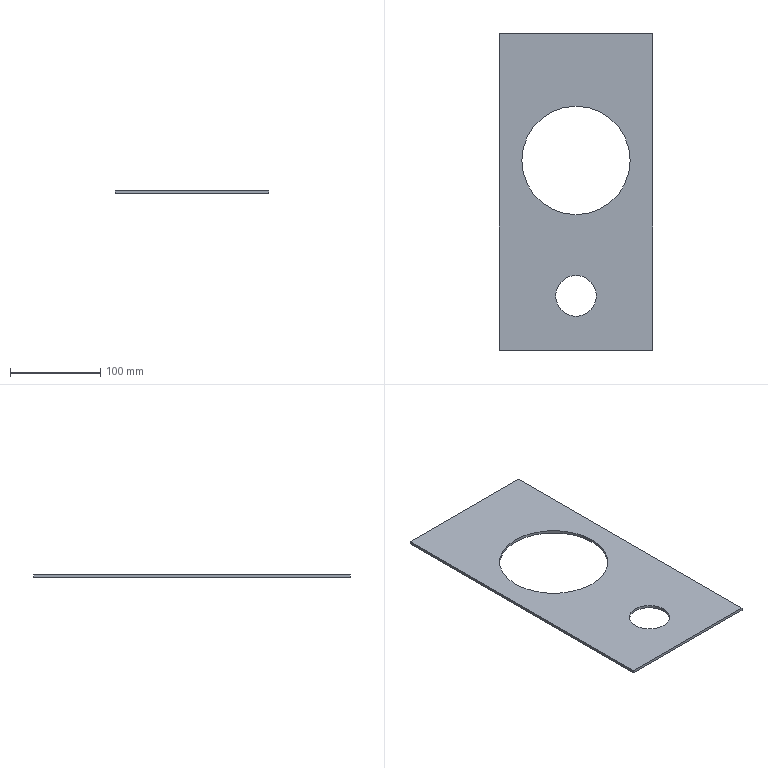Part | SolidWorks | features Extrusion 1 | 1 solid | 10 faces | box 170 x 350 x 3 mm | volume 139800 mm3 | plane 6 | cylinder 4 | commonest cylinder face diameters 45 x2 120 x2
STEP:
#1=CARTESIAN_POINT('',(62.5,60.,3.));
#2=VERTEX_POINT('',#1);
#3=CARTESIAN_POINT('',(107.5,60.,3.));
#4=VERTEX_POINT('',#3);
#5=CARTESIAN_POINT('',(85.,60.,3.));
#6=DIRECTION('',(0.,0.,1.));
#7=DIRECTION('',(1.,0.,0.));
#8=AXIS2_PLACEMENT_3D('',#5,#6,#7);
#9=CIRCLE('',#8,22.5);
#10=EDGE_CURVE('',#2,#4,#9,.T.);
#11=ORIENTED_EDGE('',*,*,#10,.T.);
#12=CARTESIAN_POINT('',(107.5,60.,0.));
#13=VERTEX_POINT('',#12);
#14=CARTESIAN_POINT('',(107.5,60.,3.));
#15=DIRECTION('',(0.,0.,-1.));
#16=VECTOR('',#15,1000.);
#17=LINE('',#14,#16);
#18=EDGE_CURVE('',#4,#13,#17,.T.);
#19=ORIENTED_EDGE('',*,*,#18,.T.);
#20=CARTESIAN_POINT('',(62.5,60.,0.));
#21=VERTEX_POINT('',#20);
#22=CARTESIAN_POINT('',(85.,60.,0.));
#23=DIRECTION('',(0.,0.,1.));
#24=DIRECTION('',(1.,0.,0.));
#25=AXIS2_PLACEMENT_3D('',#22,#23,#24);
#26=CIRCLE('',#25,22.5);
#27=EDGE_CURVE('',#21,#13,#26,.T.);
#28=ORIENTED_EDGE('',*,*,#27,.F.);
#29=CARTESIAN_POINT('',(62.5,60.,3.));
#30=DIRECTION('',(0.,0.,-1.));
#31=VECTOR('',#30,1000.);
#32=LINE('',#29,#31);
#33=EDGE_CURVE('',#2,#21,#32,.T.);
#34=ORIENTED_EDGE('',*,*,#33,.F.);
#35=EDGE_LOOP('',(#11,#19,#28,#34));
#36=FACE_OUTER_BOUND('',#35,.T.);
#37=CARTESIAN_POINT('',(85.,60.,3.));
#38=DIRECTION('',(0.,0.,-1.));
#39=DIRECTION('',(-1.,0.,0.));
#40=AXIS2_PLACEMENT_3D('',#37,#38,#39);
#41=CYLINDRICAL_SURFACE('',#40,22.5);
#42=ADVANCED_FACE('',(#36),#41,.F.);
#43=CARTESIAN_POINT('',(25.,210.,3.));
#44=VERTEX_POINT('',#43);
#45=CARTESIAN_POINT('',(145.,210.,3.));
#46=VERTEX_POINT('',#45);
#47=CARTESIAN_POINT('',(85.,210.,3.));
#48=DIRECTION('',(0.,0.,1.));
#49=DIRECTION('',(1.,0.,0.));
#50=AXIS2_PLACEMENT_3D('',#47,#48,#49);
#51=CIRCLE('',#50,60.);
#52=EDGE_CURVE('',#44,#46,#51,.T.);
#53=ORIENTED_EDGE('',*,*,#52,.T.);
#54=CARTESIAN_POINT('',(145.,210.,0.));
#55=VERTEX_POINT('',#54);
#56=CARTESIAN_POINT('',(145.,210.,3.));
#57=DIRECTION('',(0.,0.,-1.));
#58=VECTOR('',#57,1000.);
#59=LINE('',#56,#58);
#60=EDGE_CURVE('',#46,#55,#59,.T.);
#61=ORIENTED_EDGE('',*,*,#60,.T.);
#62=CARTESIAN_POINT('',(25.,210.,0.));
#63=VERTEX_POINT('',#62);
#64=CARTESIAN_POINT('',(85.,210.,0.));
#65=DIRECTION('',(0.,0.,1.));
#66=DIRECTION('',(1.,0.,0.));
#67=AXIS2_PLACEMENT_3D('',#64,#65,#66);
#68=CIRCLE('',#67,60.);
#69=EDGE_CURVE('',#63,#55,#68,.T.);
#70=ORIENTED_EDGE('',*,*,#69,.F.);
#71=CARTESIAN_POINT('',(25.,210.,3.));
#72=DIRECTION('',(0.,0.,-1.));
#73=VECTOR('',#72,1000.);
#74=LINE('',#71,#73);
#75=EDGE_CURVE('',#44,#63,#74,.T.);
#76=ORIENTED_EDGE('',*,*,#75,.F.);
#77=EDGE_LOOP('',(#53,#61,#70,#76));
#78=FACE_OUTER_BOUND('',#77,.T.);
#79=CARTESIAN_POINT('',(85.,210.,3.));
#80=DIRECTION('',(0.,0.,-1.));
#81=DIRECTION('',(-1.,0.,0.));
#82=AXIS2_PLACEMENT_3D('',#79,#80,#81);
#83=CYLINDRICAL_SURFACE('',#82,60.);
#84=ADVANCED_FACE('',(#78),#83,.F.);
#85=ORIENTED_EDGE('',*,*,#52,.F.);
#86=CARTESIAN_POINT('',(85.,210.,3.));
#87=DIRECTION('',(0.,0.,1.));
#88=DIRECTION('',(1.,0.,0.));
#89=AXIS2_PLACEMENT_3D('',#86,#87,#88);
#90=CIRCLE('',#89,60.);
#91=EDGE_CURVE('',#46,#44,#90,.T.);
#92=ORIENTED_EDGE('',*,*,#91,.F.);
#93=EDGE_LOOP('',(#85,#92));
#94=FACE_BOUND('',#93,.T.);
#95=CARTESIAN_POINT('',(0.,350.,3.));
#96=VERTEX_POINT('',#95);
#97=CARTESIAN_POINT('',(0.,0.,3.));
#98=VERTEX_POINT('',#97);
#99=CARTESIAN_POINT('',(0.,0.,3.));
#100=DIRECTION('',(0.,-1.,0.));
#101=VECTOR('',#100,1000.);
#102=LINE('',#99,#101);
#103=EDGE_CURVE('',#96,#98,#102,.T.);
#104=ORIENTED_EDGE('',*,*,#103,.T.);
#105=CARTESIAN_POINT('',(170.,0.,3.));
#106=VERTEX_POINT('',#105);
#107=CARTESIAN_POINT('',(0.,0.,3.));
#108=DIRECTION('',(1.,0.,0.));
#109=VECTOR('',#108,1000.);
#110=LINE('',#107,#109);
#111=EDGE_CURVE('',#98,#106,#110,.T.);
#112=ORIENTED_EDGE('',*,*,#111,.T.);
#113=CARTESIAN_POINT('',(170.,350.,3.));
#114=VERTEX_POINT('',#113);
#115=CARTESIAN_POINT('',(170.,0.,3.));
#116=DIRECTION('',(0.,1.,0.));
#117=VECTOR('',#116,1000.);
#118=LINE('',#115,#117);
#119=EDGE_CURVE('',#106,#114,#118,.T.);
#120=ORIENTED_EDGE('',*,*,#119,.T.);
#121=CARTESIAN_POINT('',(0.,350.,3.));
#122=DIRECTION('',(-1.,0.,0.));
#123=VECTOR('',#122,1000.);
#124=LINE('',#121,#123);
#125=EDGE_CURVE('',#114,#96,#124,.T.);
#126=ORIENTED_EDGE('',*,*,#125,.T.);
#127=EDGE_LOOP('',(#104,#112,#120,#126));
#128=FACE_OUTER_BOUND('',#127,.T.);
#129=ORIENTED_EDGE('',*,*,#10,.F.);
#130=CARTESIAN_POINT('',(85.,60.,3.));
#131=DIRECTION('',(0.,0.,1.));
#132=DIRECTION('',(1.,0.,0.));
#133=AXIS2_PLACEMENT_3D('',#130,#131,#132);
#134=CIRCLE('',#133,22.5);
#135=EDGE_CURVE('',#4,#2,#134,.T.);
#136=ORIENTED_EDGE('',*,*,#135,.F.);
#137=EDGE_LOOP('',(#129,#136));
#138=FACE_BOUND('',#137,.T.);
#139=CARTESIAN_POINT('',(0.,0.,3.));
#140=DIRECTION('',(0.,0.,-1.));
#141=DIRECTION('',(-1.,0.,0.));
#142=AXIS2_PLACEMENT_3D('',#139,#140,#141);
#143=PLANE('',#142);
#144=ADVANCED_FACE('',(#94,#128,#138),#143,.F.);
#145=ORIENTED_EDGE('',*,*,#69,.T.);
#146=CARTESIAN_POINT('',(85.,210.,0.));
#147=DIRECTION('',(0.,0.,1.));
#148=DIRECTION('',(1.,0.,0.));
#149=AXIS2_PLACEMENT_3D('',#146,#147,#148);
#150=CIRCLE('',#149,60.);
#151=EDGE_CURVE('',#55,#63,#150,.T.);
#152=ORIENTED_EDGE('',*,*,#151,.T.);
#153=EDGE_LOOP('',(#145,#152));
#154=FACE_BOUND('',#153,.T.);
#155=CARTESIAN_POINT('',(0.,350.,0.));
#156=VERTEX_POINT('',#155);
#157=CARTESIAN_POINT('',(0.,0.,0.));
#158=VERTEX_POINT('',#157);
#159=CARTESIAN_POINT('',(0.,0.,0.));
#160=DIRECTION('',(0.,-1.,0.));
#161=VECTOR('',#160,1000.);
#162=LINE('',#159,#161);
#163=EDGE_CURVE('',#156,#158,#162,.T.);
#164=ORIENTED_EDGE('',*,*,#163,.F.);
#165=CARTESIAN_POINT('',(170.,350.,0.));
#166=VERTEX_POINT('',#165);
#167=CARTESIAN_POINT('',(0.,350.,0.));
#168=DIRECTION('',(-1.,0.,0.));
#169=VECTOR('',#168,1000.);
#170=LINE('',#167,#169);
#171=EDGE_CURVE('',#166,#156,#170,.T.);
#172=ORIENTED_EDGE('',*,*,#171,.F.);
#173=CARTESIAN_POINT('',(170.,0.,0.));
#174=VERTEX_POINT('',#173);
#175=CARTESIAN_POINT('',(170.,0.,0.));
#176=DIRECTION('',(0.,1.,0.));
#177=VECTOR('',#176,1000.);
#178=LINE('',#175,#177);
#179=EDGE_CURVE('',#174,#166,#178,.T.);
#180=ORIENTED_EDGE('',*,*,#179,.F.);
#181=CARTESIAN_POINT('',(0.,0.,0.));
#182=DIRECTION('',(1.,0.,0.));
#183=VECTOR('',#182,1000.);
#184=LINE('',#181,#183);
#185=EDGE_CURVE('',#158,#174,#184,.T.);
#186=ORIENTED_EDGE('',*,*,#185,.F.);
#187=EDGE_LOOP('',(#164,#172,#180,#186));
#188=FACE_OUTER_BOUND('',#187,.T.);
#189=ORIENTED_EDGE('',*,*,#27,.T.);
#190=CARTESIAN_POINT('',(85.,60.,0.));
#191=DIRECTION('',(0.,0.,1.));
#192=DIRECTION('',(1.,0.,0.));
#193=AXIS2_PLACEMENT_3D('',#190,#191,#192);
#194=CIRCLE('',#193,22.5);
#195=EDGE_CURVE('',#13,#21,#194,.T.);
#196=ORIENTED_EDGE('',*,*,#195,.T.);
#197=EDGE_LOOP('',(#189,#196));
#198=FACE_BOUND('',#197,.T.);
#199=CARTESIAN_POINT('',(0.,0.,0.));
#200=DIRECTION('',(0.,0.,-1.));
#201=DIRECTION('',(-1.,0.,0.));
#202=AXIS2_PLACEMENT_3D('',#199,#200,#201);
#203=PLANE('',#202);
#204=ADVANCED_FACE('',(#154,#188,#198),#203,.T.);
#205=ORIENTED_EDGE('',*,*,#163,.T.);
#206=CARTESIAN_POINT('',(0.,0.,3.));
#207=DIRECTION('',(0.,0.,-1.));
#208=VECTOR('',#207,1000.);
#209=LINE('',#206,#208);
#210=EDGE_CURVE('',#98,#158,#209,.T.);
#211=ORIENTED_EDGE('',*,*,#210,.F.);
#212=ORIENTED_EDGE('',*,*,#103,.F.);
#213=CARTESIAN_POINT('',(0.,350.,3.));
#214=DIRECTION('',(0.,0.,-1.));
#215=VECTOR('',#214,1000.);
#216=LINE('',#213,#215);
#217=EDGE_CURVE('',#96,#156,#216,.T.);
#218=ORIENTED_EDGE('',*,*,#217,.T.);
#219=EDGE_LOOP('',(#205,#211,#212,#218));
#220=FACE_OUTER_BOUND('',#219,.T.);
#221=CARTESIAN_POINT('',(0.,0.,3.));
#222=DIRECTION('',(1.,0.,0.));
#223=DIRECTION('',(0.,0.,-1.));
#224=AXIS2_PLACEMENT_3D('',#221,#222,#223);
#225=PLANE('',#224);
#226=ADVANCED_FACE('',(#220),#225,.F.);
#227=ORIENTED_EDGE('',*,*,#185,.T.);
#228=CARTESIAN_POINT('',(170.,0.,3.));
#229=DIRECTION('',(0.,0.,-1.));
#230=VECTOR('',#229,1000.);
#231=LINE('',#228,#230);
#232=EDGE_CURVE('',#106,#174,#231,.T.);
#233=ORIENTED_EDGE('',*,*,#232,.F.);
#234=ORIENTED_EDGE('',*,*,#111,.F.);
#235=ORIENTED_EDGE('',*,*,#210,.T.);
#236=EDGE_LOOP('',(#227,#233,#234,#235));
#237=FACE_OUTER_BOUND('',#236,.T.);
#238=CARTESIAN_POINT('',(0.,0.,3.));
#239=DIRECTION('',(0.,1.,0.));
#240=DIRECTION('',(0.,0.,1.));
#241=AXIS2_PLACEMENT_3D('',#238,#239,#240);
#242=PLANE('',#241);
#243=ADVANCED_FACE('',(#237),#242,.F.);
#244=ORIENTED_EDGE('',*,*,#179,.T.);
#245=CARTESIAN_POINT('',(170.,350.,3.));
#246=DIRECTION('',(0.,0.,-1.));
#247=VECTOR('',#246,1000.);
#248=LINE('',#245,#247);
#249=EDGE_CURVE('',#114,#166,#248,.T.);
#250=ORIENTED_EDGE('',*,*,#249,.F.);
#251=ORIENTED_EDGE('',*,*,#119,.F.);
#252=ORIENTED_EDGE('',*,*,#232,.T.);
#253=EDGE_LOOP('',(#244,#250,#251,#252));
#254=FACE_OUTER_BOUND('',#253,.T.);
#255=CARTESIAN_POINT('',(170.,0.,3.));
#256=DIRECTION('',(-1.,0.,0.));
#257=DIRECTION('',(0.,0.,1.));
#258=AXIS2_PLACEMENT_3D('',#255,#256,#257);
#259=PLANE('',#258);
#260=ADVANCED_FACE('',(#254),#259,.F.);
#261=ORIENTED_EDGE('',*,*,#171,.T.);
#262=ORIENTED_EDGE('',*,*,#217,.F.);
#263=ORIENTED_EDGE('',*,*,#125,.F.);
#264=ORIENTED_EDGE('',*,*,#249,.T.);
#265=EDGE_LOOP('',(#261,#262,#263,#264));
#266=FACE_OUTER_BOUND('',#265,.T.);
#267=CARTESIAN_POINT('',(0.,350.,3.));
#268=DIRECTION('',(0.,-1.,0.));
#269=DIRECTION('',(0.,0.,-1.));
#270=AXIS2_PLACEMENT_3D('',#267,#268,#269);
#271=PLANE('',#270);
#272=ADVANCED_FACE('',(#266),#271,.F.);
#273=ORIENTED_EDGE('',*,*,#60,.F.);
#274=ORIENTED_EDGE('',*,*,#91,.T.);
#275=ORIENTED_EDGE('',*,*,#75,.T.);
#276=ORIENTED_EDGE('',*,*,#151,.F.);
#277=EDGE_LOOP('',(#273,#274,#275,#276));
#278=FACE_OUTER_BOUND('',#277,.T.);
#279=CARTESIAN_POINT('',(85.,210.,3.));
#280=DIRECTION('',(0.,0.,-1.));
#281=DIRECTION('',(-1.,0.,0.));
#282=AXIS2_PLACEMENT_3D('',#279,#280,#281);
#283=CYLINDRICAL_SURFACE('',#282,60.);
#284=ADVANCED_FACE('',(#278),#283,.F.);
#285=ORIENTED_EDGE('',*,*,#18,.F.);
#286=ORIENTED_EDGE('',*,*,#135,.T.);
#287=ORIENTED_EDGE('',*,*,#33,.T.);
#288=ORIENTED_EDGE('',*,*,#195,.F.);
#289=EDGE_LOOP('',(#285,#286,#287,#288));
#290=FACE_OUTER_BOUND('',#289,.T.);
#291=CARTESIAN_POINT('',(85.,60.,3.));
#292=DIRECTION('',(0.,0.,-1.));
#293=DIRECTION('',(-1.,0.,0.));
#294=AXIS2_PLACEMENT_3D('',#291,#292,#293);
#295=CYLINDRICAL_SURFACE('',#294,22.5);
#296=ADVANCED_FACE('',(#290),#295,.F.);
#297=CLOSED_SHELL('',(#42,#84,#144,#204,#226,#243,#260,#272,#284,#296));
#298=MANIFOLD_SOLID_BREP('',#297);
#299=CARTESIAN_POINT('',(0.,0.,0.));
#300=DIRECTION('',(0.,0.,1.));
#301=DIRECTION('',(1.,0.,0.));
#302=AXIS2_PLACEMENT_3D('',#299,#300,#301);
#303=(LENGTH_UNIT()NAMED_UNIT(*)SI_UNIT(.MILLI.,.METRE.));
#304=UNCERTAINTY_MEASURE_WITH_UNIT(LENGTH_MEASURE(0.00001),#303,'','');
#305=(NAMED_UNIT(*)PLANE_ANGLE_UNIT()SI_UNIT($,.RADIAN.));
#306=(NAMED_UNIT(*)SI_UNIT($,.STERADIAN.)SOLID_ANGLE_UNIT());
#307=(GEOMETRIC_REPRESENTATION_CONTEXT(3)GLOBAL_UNCERTAINTY_ASSIGNED_CONTEXT((#304))GLOBAL_UNIT_ASSIGNED_CONTEXT((#303,#305,#306))REPRESENTATION_CONTEXT('',''));
#308=ADVANCED_BREP_SHAPE_REPRESENTATION('',(#298,#302),#307);